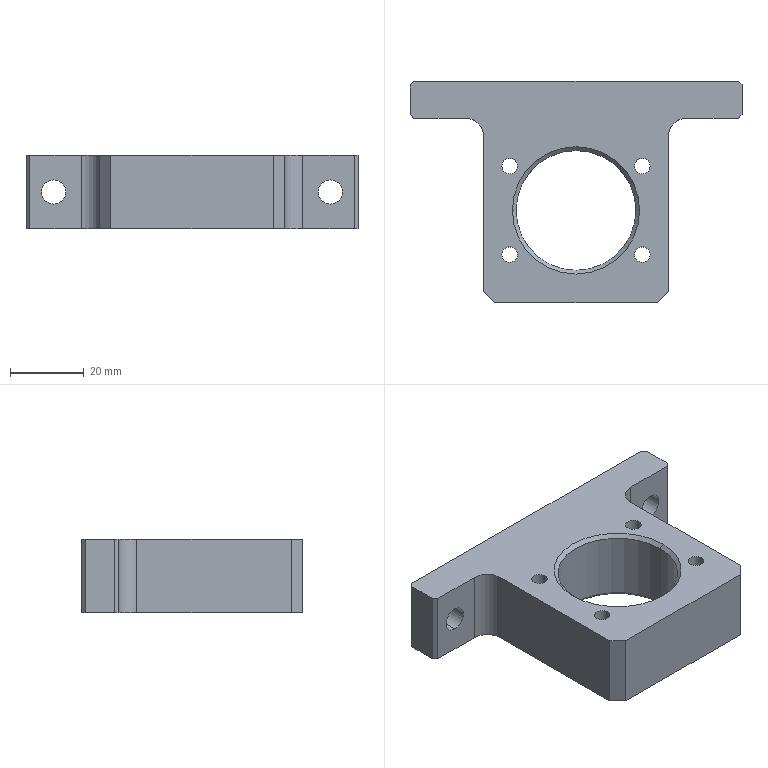Part | STEP file | linear bearing mounting plate | 1 solid | 36 faces | box 90 x 60 x 20 mm | volume 49506 mm3 | cylinder 16 | plane 16 | cone 4 | commonest cylinder face diameters 4.2 x8 6.6 x4 10 x2 32.5 x2